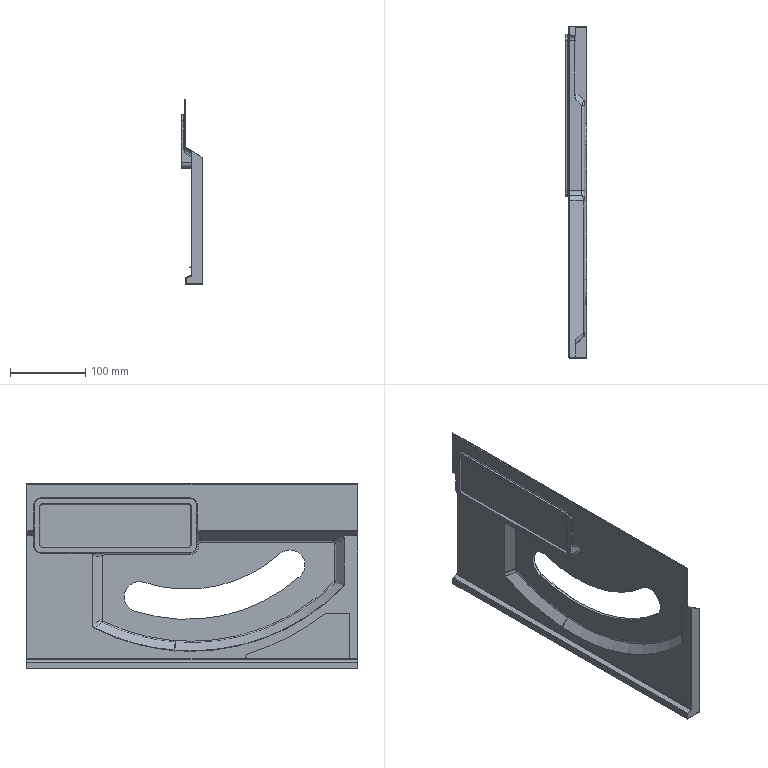Part | STEP file | DEWALT-DWE7492-B22 | 1 solid | 184 faces | box 29 x 440 x 245 mm | volume 127780 mm3 | plane 66 | cylinder 61 | spline 33 | torus 12 | cone 11 | sphere 1 | commonest cylinder face diameters 2 x19 4 x8 14 x7 6 x6 8 x5 16 x4